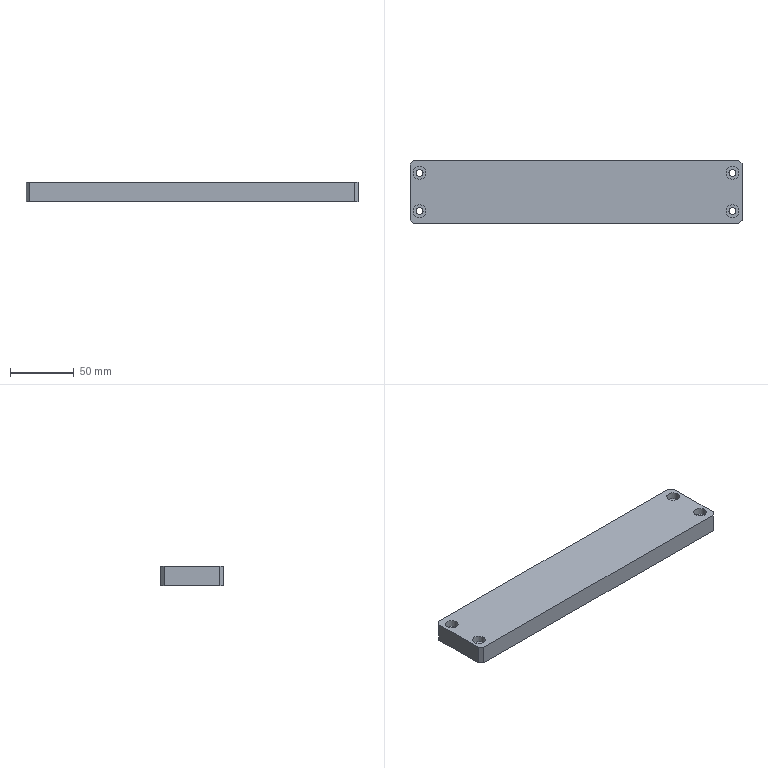Part | NX | 1 solid | 22 faces | box 261 x 50 x 15 mm | volume 192871 mm3 | plane 14 | cylinder 8 | commonest cylinder face diameters 5.5 x4 10 x4
STEP:
#1=CARTESIAN_POINT('',(-127.5,25.,7.5));
#2=VERTEX_POINT('',#1);
#3=CARTESIAN_POINT('',(-130.5,22.,7.5));
#4=VERTEX_POINT('',#3);
#5=CARTESIAN_POINT('',(-130.5,22.,7.5));
#6=DIRECTION('',(-0.7071,-0.7071,0.));
#7=VECTOR('',#6,1000.);
#8=LINE('',#5,#7);
#9=EDGE_CURVE('',#2,#4,#8,.T.);
#10=ORIENTED_EDGE('',*,*,#9,.F.);
#11=CARTESIAN_POINT('',(-127.5,25.,-7.5));
#12=VERTEX_POINT('',#11);
#13=CARTESIAN_POINT('',(-127.5,25.,7.5));
#14=DIRECTION('',(0.,0.,1.));
#15=VECTOR('',#14,1000.);
#16=LINE('',#13,#15);
#17=EDGE_CURVE('',#12,#2,#16,.T.);
#18=ORIENTED_EDGE('',*,*,#17,.F.);
#19=CARTESIAN_POINT('',(-130.5,22.,-7.5));
#20=VERTEX_POINT('',#19);
#21=CARTESIAN_POINT('',(-76.25,76.25,-7.5));
#22=DIRECTION('',(0.7071,0.7071,0.));
#23=VECTOR('',#22,1000.);
#24=LINE('',#21,#23);
#25=EDGE_CURVE('',#20,#12,#24,.T.);
#26=ORIENTED_EDGE('',*,*,#25,.F.);
#27=CARTESIAN_POINT('',(-130.5,22.,7.5));
#28=DIRECTION('',(0.,0.,-1.));
#29=VECTOR('',#28,1000.);
#30=LINE('',#27,#29);
#31=EDGE_CURVE('',#4,#20,#30,.T.);
#32=ORIENTED_EDGE('',*,*,#31,.F.);
#33=EDGE_LOOP('',(#10,#18,#26,#32));
#34=FACE_BOUND('',#33,.T.);
#35=CARTESIAN_POINT('',(-130.5,22.,7.5));
#36=DIRECTION('',(0.7071,-0.7071,0.));
#37=DIRECTION('',(0.,0.,-1.));
#38=AXIS2_PLACEMENT_3D('',#35,#36,#37);
#39=PLANE('',#38);
#40=ADVANCED_FACE('',(#34),#39,.F.);
#41=CARTESIAN_POINT('',(-130.5,-22.,7.5));
#42=VERTEX_POINT('',#41);
#43=CARTESIAN_POINT('',(-127.5,-25.,7.5));
#44=VERTEX_POINT('',#43);
#45=CARTESIAN_POINT('',(-127.5,-25.,7.5));
#46=DIRECTION('',(0.7071,-0.7071,0.));
#47=VECTOR('',#46,1000.);
#48=LINE('',#45,#47);
#49=EDGE_CURVE('',#42,#44,#48,.T.);
#50=ORIENTED_EDGE('',*,*,#49,.F.);
#51=CARTESIAN_POINT('',(-130.5,-22.,-7.5));
#52=VERTEX_POINT('',#51);
#53=CARTESIAN_POINT('',(-130.5,-22.,7.5));
#54=DIRECTION('',(0.,0.,1.));
#55=VECTOR('',#54,1000.);
#56=LINE('',#53,#55);
#57=EDGE_CURVE('',#52,#42,#56,.T.);
#58=ORIENTED_EDGE('',*,*,#57,.F.);
#59=CARTESIAN_POINT('',(-127.5,-25.,-7.5));
#60=VERTEX_POINT('',#59);
#61=CARTESIAN_POINT('',(-76.25,-76.25,-7.5));
#62=DIRECTION('',(-0.7071,0.7071,0.));
#63=VECTOR('',#62,1000.);
#64=LINE('',#61,#63);
#65=EDGE_CURVE('',#60,#52,#64,.T.);
#66=ORIENTED_EDGE('',*,*,#65,.F.);
#67=CARTESIAN_POINT('',(-127.5,-25.,-7.5));
#68=DIRECTION('',(0.,0.,-1.));
#69=VECTOR('',#68,1000.);
#70=LINE('',#67,#69);
#71=EDGE_CURVE('',#44,#60,#70,.T.);
#72=ORIENTED_EDGE('',*,*,#71,.F.);
#73=EDGE_LOOP('',(#50,#58,#66,#72));
#74=FACE_BOUND('',#73,.T.);
#75=CARTESIAN_POINT('',(-127.5,-25.,7.5));
#76=DIRECTION('',(-0.7071,-0.7071,0.));
#77=DIRECTION('',(0.,0.,1.));
#78=AXIS2_PLACEMENT_3D('',#75,#76,#77);
#79=PLANE('',#78);
#80=ADVANCED_FACE('',(#74),#79,.T.);
#81=CARTESIAN_POINT('',(130.5,22.,7.5));
#82=VERTEX_POINT('',#81);
#83=CARTESIAN_POINT('',(127.5,25.,7.5));
#84=VERTEX_POINT('',#83);
#85=CARTESIAN_POINT('',(127.5,25.,7.5));
#86=DIRECTION('',(-0.7071,0.7071,0.));
#87=VECTOR('',#86,1000.);
#88=LINE('',#85,#87);
#89=EDGE_CURVE('',#82,#84,#88,.T.);
#90=ORIENTED_EDGE('',*,*,#89,.F.);
#91=CARTESIAN_POINT('',(130.5,22.,-7.5));
#92=VERTEX_POINT('',#91);
#93=CARTESIAN_POINT('',(130.5,22.,7.5));
#94=DIRECTION('',(0.,0.,1.));
#95=VECTOR('',#94,1000.);
#96=LINE('',#93,#95);
#97=EDGE_CURVE('',#92,#82,#96,.T.);
#98=ORIENTED_EDGE('',*,*,#97,.F.);
#99=CARTESIAN_POINT('',(127.5,25.,-7.5));
#100=VERTEX_POINT('',#99);
#101=CARTESIAN_POINT('',(76.25,76.25,-7.5));
#102=DIRECTION('',(0.7071,-0.7071,0.));
#103=VECTOR('',#102,1000.);
#104=LINE('',#101,#103);
#105=EDGE_CURVE('',#100,#92,#104,.T.);
#106=ORIENTED_EDGE('',*,*,#105,.F.);
#107=CARTESIAN_POINT('',(127.5,25.,-7.5));
#108=DIRECTION('',(0.,0.,-1.));
#109=VECTOR('',#108,1000.);
#110=LINE('',#107,#109);
#111=EDGE_CURVE('',#84,#100,#110,.T.);
#112=ORIENTED_EDGE('',*,*,#111,.F.);
#113=EDGE_LOOP('',(#90,#98,#106,#112));
#114=FACE_BOUND('',#113,.T.);
#115=CARTESIAN_POINT('',(127.5,25.,7.5));
#116=DIRECTION('',(0.7071,0.7071,0.));
#117=DIRECTION('',(0.,0.,1.));
#118=AXIS2_PLACEMENT_3D('',#115,#116,#117);
#119=PLANE('',#118);
#120=ADVANCED_FACE('',(#114),#119,.T.);
#121=CARTESIAN_POINT('',(127.5,-25.,7.5));
#122=VERTEX_POINT('',#121);
#123=CARTESIAN_POINT('',(130.5,-22.,7.5));
#124=VERTEX_POINT('',#123);
#125=CARTESIAN_POINT('',(130.5,-22.,7.5));
#126=DIRECTION('',(0.7071,0.7071,0.));
#127=VECTOR('',#126,1000.);
#128=LINE('',#125,#127);
#129=EDGE_CURVE('',#122,#124,#128,.T.);
#130=ORIENTED_EDGE('',*,*,#129,.F.);
#131=CARTESIAN_POINT('',(127.5,-25.,-7.5));
#132=VERTEX_POINT('',#131);
#133=CARTESIAN_POINT('',(127.5,-25.,7.5));
#134=DIRECTION('',(0.,0.,1.));
#135=VECTOR('',#134,1000.);
#136=LINE('',#133,#135);
#137=EDGE_CURVE('',#132,#122,#136,.T.);
#138=ORIENTED_EDGE('',*,*,#137,.F.);
#139=CARTESIAN_POINT('',(130.5,-22.,-7.5));
#140=VERTEX_POINT('',#139);
#141=CARTESIAN_POINT('',(76.25,-76.25,-7.5));
#142=DIRECTION('',(-0.7071,-0.7071,0.));
#143=VECTOR('',#142,1000.);
#144=LINE('',#141,#143);
#145=EDGE_CURVE('',#140,#132,#144,.T.);
#146=ORIENTED_EDGE('',*,*,#145,.F.);
#147=CARTESIAN_POINT('',(130.5,-22.,7.5));
#148=DIRECTION('',(0.,0.,-1.));
#149=VECTOR('',#148,1000.);
#150=LINE('',#147,#149);
#151=EDGE_CURVE('',#124,#140,#150,.T.);
#152=ORIENTED_EDGE('',*,*,#151,.F.);
#153=EDGE_LOOP('',(#130,#138,#146,#152));
#154=FACE_BOUND('',#153,.T.);
#155=CARTESIAN_POINT('',(130.5,-22.,7.5));
#156=DIRECTION('',(-0.7071,0.7071,0.));
#157=DIRECTION('',(0.,0.,-1.));
#158=AXIS2_PLACEMENT_3D('',#155,#156,#157);
#159=PLANE('',#158);
#160=ADVANCED_FACE('',(#154),#159,.F.);
#161=CARTESIAN_POINT('',(128.,15.,2.1));
#162=VERTEX_POINT('',#161);
#163=CARTESIAN_POINT('',(123.,15.,2.1));
#164=DIRECTION('',(0.,0.,1.));
#165=DIRECTION('',(1.,0.,0.));
#166=AXIS2_PLACEMENT_3D('',#163,#164,#165);
#167=CIRCLE('',#166,5.);
#168=EDGE_CURVE('',#162,#162,#167,.T.);
#169=ORIENTED_EDGE('',*,*,#168,.T.);
#170=EDGE_LOOP('',(#169));
#171=FACE_BOUND('',#170,.T.);
#172=CARTESIAN_POINT('',(125.75,15.,2.1));
#173=VERTEX_POINT('',#172);
#174=CARTESIAN_POINT('',(123.,15.,2.1));
#175=DIRECTION('',(0.,0.,1.));
#176=DIRECTION('',(1.,0.,0.));
#177=AXIS2_PLACEMENT_3D('',#174,#175,#176);
#178=CIRCLE('',#177,2.75);
#179=EDGE_CURVE('',#173,#173,#178,.T.);
#180=ORIENTED_EDGE('',*,*,#179,.F.);
#181=EDGE_LOOP('',(#180));
#182=FACE_BOUND('',#181,.T.);
#183=CARTESIAN_POINT('',(125.75,15.,2.1));
#184=DIRECTION('',(0.,0.,-1.));
#185=DIRECTION('',(-1.,0.,0.));
#186=AXIS2_PLACEMENT_3D('',#183,#184,#185);
#187=PLANE('',#186);
#188=ADVANCED_FACE('',(#171,#182),#187,.F.);
#189=CARTESIAN_POINT('',(118.,-15.,2.1));
#190=VERTEX_POINT('',#189);
#191=CARTESIAN_POINT('',(123.,-15.,2.1));
#192=DIRECTION('',(0.,0.,1.));
#193=DIRECTION('',(-1.,0.,0.));
#194=AXIS2_PLACEMENT_3D('',#191,#192,#193);
#195=CIRCLE('',#194,5.);
#196=EDGE_CURVE('',#190,#190,#195,.T.);
#197=ORIENTED_EDGE('',*,*,#196,.T.);
#198=EDGE_LOOP('',(#197));
#199=FACE_BOUND('',#198,.T.);
#200=CARTESIAN_POINT('',(120.25,-15.,2.1));
#201=VERTEX_POINT('',#200);
#202=CARTESIAN_POINT('',(123.,-15.,2.1));
#203=DIRECTION('',(0.,0.,1.));
#204=DIRECTION('',(-1.,0.,0.));
#205=AXIS2_PLACEMENT_3D('',#202,#203,#204);
#206=CIRCLE('',#205,2.75);
#207=EDGE_CURVE('',#201,#201,#206,.T.);
#208=ORIENTED_EDGE('',*,*,#207,.F.);
#209=EDGE_LOOP('',(#208));
#210=FACE_BOUND('',#209,.T.);
#211=CARTESIAN_POINT('',(125.75,15.,2.1));
#212=DIRECTION('',(0.,0.,-1.));
#213=DIRECTION('',(-1.,0.,0.));
#214=AXIS2_PLACEMENT_3D('',#211,#212,#213);
#215=PLANE('',#214);
#216=ADVANCED_FACE('',(#199,#210),#215,.F.);
#217=CARTESIAN_POINT('',(-128.,15.,2.1));
#218=VERTEX_POINT('',#217);
#219=CARTESIAN_POINT('',(-123.,15.,2.1));
#220=DIRECTION('',(0.,0.,1.));
#221=DIRECTION('',(-1.,0.,0.));
#222=AXIS2_PLACEMENT_3D('',#219,#220,#221);
#223=CIRCLE('',#222,5.);
#224=EDGE_CURVE('',#218,#218,#223,.T.);
#225=ORIENTED_EDGE('',*,*,#224,.T.);
#226=EDGE_LOOP('',(#225));
#227=FACE_BOUND('',#226,.T.);
#228=CARTESIAN_POINT('',(-125.75,15.,2.1));
#229=VERTEX_POINT('',#228);
#230=CARTESIAN_POINT('',(-123.,15.,2.1));
#231=DIRECTION('',(0.,0.,1.));
#232=DIRECTION('',(-1.,0.,0.));
#233=AXIS2_PLACEMENT_3D('',#230,#231,#232);
#234=CIRCLE('',#233,2.75);
#235=EDGE_CURVE('',#229,#229,#234,.T.);
#236=ORIENTED_EDGE('',*,*,#235,.F.);
#237=EDGE_LOOP('',(#236));
#238=FACE_BOUND('',#237,.T.);
#239=CARTESIAN_POINT('',(125.75,15.,2.1));
#240=DIRECTION('',(0.,0.,-1.));
#241=DIRECTION('',(-1.,0.,0.));
#242=AXIS2_PLACEMENT_3D('',#239,#240,#241);
#243=PLANE('',#242);
#244=ADVANCED_FACE('',(#227,#238),#243,.F.);
#245=CARTESIAN_POINT('',(-128.,-15.,2.1));
#246=VERTEX_POINT('',#245);
#247=CARTESIAN_POINT('',(-123.,-15.,2.1));
#248=DIRECTION('',(0.,0.,1.));
#249=DIRECTION('',(-1.,0.,0.));
#250=AXIS2_PLACEMENT_3D('',#247,#248,#249);
#251=CIRCLE('',#250,5.);
#252=EDGE_CURVE('',#246,#246,#251,.T.);
#253=ORIENTED_EDGE('',*,*,#252,.T.);
#254=EDGE_LOOP('',(#253));
#255=FACE_BOUND('',#254,.T.);
#256=CARTESIAN_POINT('',(-125.75,-15.,2.1));
#257=VERTEX_POINT('',#256);
#258=CARTESIAN_POINT('',(-123.,-15.,2.1));
#259=DIRECTION('',(0.,0.,1.));
#260=DIRECTION('',(-1.,0.,0.));
#261=AXIS2_PLACEMENT_3D('',#258,#259,#260);
#262=CIRCLE('',#261,2.75);
#263=EDGE_CURVE('',#257,#257,#262,.T.);
#264=ORIENTED_EDGE('',*,*,#263,.F.);
#265=EDGE_LOOP('',(#264));
#266=FACE_BOUND('',#265,.T.);
#267=CARTESIAN_POINT('',(125.75,15.,2.1));
#268=DIRECTION('',(0.,0.,-1.));
#269=DIRECTION('',(-1.,0.,0.));
#270=AXIS2_PLACEMENT_3D('',#267,#268,#269);
#271=PLANE('',#270);
#272=ADVANCED_FACE('',(#255,#266),#271,.F.);
#273=CARTESIAN_POINT('',(130.5,-25.,-7.5));
#274=DIRECTION('',(0.,1.,0.));
#275=VECTOR('',#274,1000.);
#276=LINE('',#273,#275);
#277=EDGE_CURVE('',#140,#92,#276,.T.);
#278=ORIENTED_EDGE('',*,*,#277,.F.);
#279=ORIENTED_EDGE('',*,*,#145,.T.);
#280=CARTESIAN_POINT('',(-130.5,-25.,-7.5));
#281=DIRECTION('',(1.,0.,0.));
#282=VECTOR('',#281,1000.);
#283=LINE('',#280,#282);
#284=EDGE_CURVE('',#60,#132,#283,.T.);
#285=ORIENTED_EDGE('',*,*,#284,.F.);
#286=ORIENTED_EDGE('',*,*,#65,.T.);
#287=CARTESIAN_POINT('',(-130.5,-25.,-7.5));
#288=DIRECTION('',(0.,1.,0.));
#289=VECTOR('',#288,1000.);
#290=LINE('',#287,#289);
#291=EDGE_CURVE('',#52,#20,#290,.T.);
#292=ORIENTED_EDGE('',*,*,#291,.T.);
#293=ORIENTED_EDGE('',*,*,#25,.T.);
#294=CARTESIAN_POINT('',(-130.5,25.,-7.5));
#295=DIRECTION('',(1.,0.,0.));
#296=VECTOR('',#295,1000.);
#297=LINE('',#294,#296);
#298=EDGE_CURVE('',#12,#100,#297,.T.);
#299=ORIENTED_EDGE('',*,*,#298,.T.);
#300=ORIENTED_EDGE('',*,*,#105,.T.);
#301=EDGE_LOOP('',(#278,#279,#285,#286,#292,#293,#299,#300));
#302=FACE_BOUND('',#301,.T.);
#303=CARTESIAN_POINT('',(-120.25,-15.,-7.5));
#304=VERTEX_POINT('',#303);
#305=CARTESIAN_POINT('',(-123.,-15.,-7.5));
#306=DIRECTION('',(0.,0.,1.));
#307=DIRECTION('',(1.,0.,0.));
#308=AXIS2_PLACEMENT_3D('',#305,#306,#307);
#309=CIRCLE('',#308,2.75);
#310=EDGE_CURVE('',#304,#304,#309,.T.);
#311=ORIENTED_EDGE('',*,*,#310,.T.);
#312=EDGE_LOOP('',(#311));
#313=FACE_BOUND('',#312,.T.);
#314=CARTESIAN_POINT('',(-120.25,15.,-7.5));
#315=VERTEX_POINT('',#314);
#316=CARTESIAN_POINT('',(-123.,15.,-7.5));
#317=DIRECTION('',(0.,0.,1.));
#318=DIRECTION('',(1.,0.,0.));
#319=AXIS2_PLACEMENT_3D('',#316,#317,#318);
#320=CIRCLE('',#319,2.75);
#321=EDGE_CURVE('',#315,#315,#320,.T.);
#322=ORIENTED_EDGE('',*,*,#321,.T.);
#323=EDGE_LOOP('',(#322));
#324=FACE_BOUND('',#323,.T.);
#325=CARTESIAN_POINT('',(125.75,-15.,-7.5));
#326=VERTEX_POINT('',#325);
#327=CARTESIAN_POINT('',(123.,-15.,-7.5));
#328=DIRECTION('',(0.,0.,1.));
#329=DIRECTION('',(1.,0.,0.));
#330=AXIS2_PLACEMENT_3D('',#327,#328,#329);
#331=CIRCLE('',#330,2.75);
#332=EDGE_CURVE('',#326,#326,#331,.T.);
#333=ORIENTED_EDGE('',*,*,#332,.T.);
#334=EDGE_LOOP('',(#333));
#335=FACE_BOUND('',#334,.T.);
#336=CARTESIAN_POINT('',(125.75,15.,-7.5));
#337=VERTEX_POINT('',#336);
#338=CARTESIAN_POINT('',(123.,15.,-7.5));
#339=DIRECTION('',(0.,0.,1.));
#340=DIRECTION('',(1.,0.,0.));
#341=AXIS2_PLACEMENT_3D('',#338,#339,#340);
#342=CIRCLE('',#341,2.75);
#343=EDGE_CURVE('',#337,#337,#342,.T.);
#344=ORIENTED_EDGE('',*,*,#343,.T.);
#345=EDGE_LOOP('',(#344));
#346=FACE_BOUND('',#345,.T.);
#347=CARTESIAN_POINT('',(0.,0.,-7.5));
#348=DIRECTION('',(0.,0.,-1.));
#349=DIRECTION('',(-1.,0.,0.));
#350=AXIS2_PLACEMENT_3D('',#347,#348,#349);
#351=PLANE('',#350);
#352=ADVANCED_FACE('',(#302,#313,#324,#335,#346),#351,.T.);
#353=CARTESIAN_POINT('',(-130.5,-25.,7.5));
#354=DIRECTION('',(1.,0.,0.));
#355=VECTOR('',#354,1000.);
#356=LINE('',#353,#355);
#357=EDGE_CURVE('',#44,#122,#356,.T.);
#358=ORIENTED_EDGE('',*,*,#357,.T.);
#359=ORIENTED_EDGE('',*,*,#129,.T.);
#360=CARTESIAN_POINT('',(130.5,-25.,7.5));
#361=DIRECTION('',(0.,1.,0.));
#362=VECTOR('',#361,1000.);
#363=LINE('',#360,#362);
#364=EDGE_CURVE('',#124,#82,#363,.T.);
#365=ORIENTED_EDGE('',*,*,#364,.T.);
#366=ORIENTED_EDGE('',*,*,#89,.T.);
#367=CARTESIAN_POINT('',(-130.5,25.,7.5));
#368=DIRECTION('',(1.,0.,0.));
#369=VECTOR('',#368,1000.);
#370=LINE('',#367,#369);
#371=EDGE_CURVE('',#2,#84,#370,.T.);
#372=ORIENTED_EDGE('',*,*,#371,.F.);
#373=ORIENTED_EDGE('',*,*,#9,.T.);
#374=CARTESIAN_POINT('',(-130.5,-25.,7.5));
#375=DIRECTION('',(0.,1.,0.));
#376=VECTOR('',#375,1000.);
#377=LINE('',#374,#376);
#378=EDGE_CURVE('',#42,#4,#377,.T.);
#379=ORIENTED_EDGE('',*,*,#378,.F.);
#380=ORIENTED_EDGE('',*,*,#49,.T.);
#381=EDGE_LOOP('',(#358,#359,#365,#366,#372,#373,#379,#380));
#382=FACE_BOUND('',#381,.T.);
#383=CARTESIAN_POINT('',(-118.,-15.,7.5));
#384=VERTEX_POINT('',#383);
#385=CARTESIAN_POINT('',(-123.,-15.,7.5));
#386=DIRECTION('',(0.,0.,1.));
#387=DIRECTION('',(1.,0.,0.));
#388=AXIS2_PLACEMENT_3D('',#385,#386,#387);
#389=CIRCLE('',#388,5.);
#390=EDGE_CURVE('',#384,#384,#389,.T.);
#391=ORIENTED_EDGE('',*,*,#390,.F.);
#392=EDGE_LOOP('',(#391));
#393=FACE_BOUND('',#392,.T.);
#394=CARTESIAN_POINT('',(-118.,15.,7.5));
#395=VERTEX_POINT('',#394);
#396=CARTESIAN_POINT('',(-123.,15.,7.5));
#397=DIRECTION('',(0.,0.,1.));
#398=DIRECTION('',(1.,0.,0.));
#399=AXIS2_PLACEMENT_3D('',#396,#397,#398);
#400=CIRCLE('',#399,5.);
#401=EDGE_CURVE('',#395,#395,#400,.T.);
#402=ORIENTED_EDGE('',*,*,#401,.F.);
#403=EDGE_LOOP('',(#402));
#404=FACE_BOUND('',#403,.T.);
#405=CARTESIAN_POINT('',(128.,-15.,7.5));
#406=VERTEX_POINT('',#405);
#407=CARTESIAN_POINT('',(123.,-15.,7.5));
#408=DIRECTION('',(0.,0.,1.));
#409=DIRECTION('',(1.,0.,0.));
#410=AXIS2_PLACEMENT_3D('',#407,#408,#409);
#411=CIRCLE('',#410,5.);
#412=EDGE_CURVE('',#406,#406,#411,.T.);
#413=ORIENTED_EDGE('',*,*,#412,.F.);
#414=EDGE_LOOP('',(#413));
#415=FACE_BOUND('',#414,.T.);
#416=CARTESIAN_POINT('',(128.,15.,7.5));
#417=VERTEX_POINT('',#416);
#418=CARTESIAN_POINT('',(123.,15.,7.5));
#419=DIRECTION('',(0.,0.,1.));
#420=DIRECTION('',(1.,0.,0.));
#421=AXIS2_PLACEMENT_3D('',#418,#419,#420);
#422=CIRCLE('',#421,5.);
#423=EDGE_CURVE('',#417,#417,#422,.T.);
#424=ORIENTED_EDGE('',*,*,#423,.F.);
#425=EDGE_LOOP('',(#424));
#426=FACE_BOUND('',#425,.T.);
#427=CARTESIAN_POINT('',(0.,0.,7.5));
#428=DIRECTION('',(0.,0.,-1.));
#429=DIRECTION('',(-1.,0.,0.));
#430=AXIS2_PLACEMENT_3D('',#427,#428,#429);
#431=PLANE('',#430);
#432=ADVANCED_FACE('',(#382,#393,#404,#415,#426),#431,.F.);
#433=ORIENTED_EDGE('',*,*,#371,.T.);
#434=ORIENTED_EDGE('',*,*,#111,.T.);
#435=ORIENTED_EDGE('',*,*,#298,.F.);
#436=ORIENTED_EDGE('',*,*,#17,.T.);
#437=EDGE_LOOP('',(#433,#434,#435,#436));
#438=FACE_BOUND('',#437,.T.);
#439=CARTESIAN_POINT('',(-130.5,25.,7.5));
#440=DIRECTION('',(0.,1.,0.));
#441=DIRECTION('',(0.,0.,1.));
#442=AXIS2_PLACEMENT_3D('',#439,#440,#441);
#443=PLANE('',#442);
#444=ADVANCED_FACE('',(#438),#443,.T.);
#445=ORIENTED_EDGE('',*,*,#364,.F.);
#446=ORIENTED_EDGE('',*,*,#151,.T.);
#447=ORIENTED_EDGE('',*,*,#277,.T.);
#448=ORIENTED_EDGE('',*,*,#97,.T.);
#449=EDGE_LOOP('',(#445,#446,#447,#448));
#450=FACE_BOUND('',#449,.T.);
#451=CARTESIAN_POINT('',(130.5,-25.,7.5));
#452=DIRECTION('',(-1.,0.,0.));
#453=DIRECTION('',(0.,0.,1.));
#454=AXIS2_PLACEMENT_3D('',#451,#452,#453);
#455=PLANE('',#454);
#456=ADVANCED_FACE('',(#450),#455,.F.);
#457=ORIENTED_EDGE('',*,*,#284,.T.);
#458=ORIENTED_EDGE('',*,*,#137,.T.);
#459=ORIENTED_EDGE('',*,*,#357,.F.);
#460=ORIENTED_EDGE('',*,*,#71,.T.);
#461=EDGE_LOOP('',(#457,#458,#459,#460));
#462=FACE_BOUND('',#461,.T.);
#463=CARTESIAN_POINT('',(-130.5,-25.,7.5));
#464=DIRECTION('',(0.,1.,0.));
#465=DIRECTION('',(0.,0.,1.));
#466=AXIS2_PLACEMENT_3D('',#463,#464,#465);
#467=PLANE('',#466);
#468=ADVANCED_FACE('',(#462),#467,.F.);
#469=ORIENTED_EDGE('',*,*,#291,.F.);
#470=ORIENTED_EDGE('',*,*,#57,.T.);
#471=ORIENTED_EDGE('',*,*,#378,.T.);
#472=ORIENTED_EDGE('',*,*,#31,.T.);
#473=EDGE_LOOP('',(#469,#470,#471,#472));
#474=FACE_BOUND('',#473,.T.);
#475=CARTESIAN_POINT('',(-130.5,-25.,7.5));
#476=DIRECTION('',(-1.,0.,0.));
#477=DIRECTION('',(0.,0.,1.));
#478=AXIS2_PLACEMENT_3D('',#475,#476,#477);
#479=PLANE('',#478);
#480=ADVANCED_FACE('',(#474),#479,.T.);
#481=ORIENTED_EDGE('',*,*,#310,.F.);
#482=EDGE_LOOP('',(#481));
#483=FACE_BOUND('',#482,.T.);
#484=ORIENTED_EDGE('',*,*,#263,.T.);
#485=EDGE_LOOP('',(#484));
#486=FACE_BOUND('',#485,.T.);
#487=CARTESIAN_POINT('',(-123.,-15.,7.5));
#488=DIRECTION('',(0.,0.,1.));
#489=DIRECTION('',(1.,0.,0.));
#490=AXIS2_PLACEMENT_3D('',#487,#488,#489);
#491=CYLINDRICAL_SURFACE('',#490,2.75);
#492=ADVANCED_FACE('',(#483,#486),#491,.F.);
#493=ORIENTED_EDGE('',*,*,#252,.F.);
#494=EDGE_LOOP('',(#493));
#495=FACE_BOUND('',#494,.T.);
#496=ORIENTED_EDGE('',*,*,#390,.T.);
#497=EDGE_LOOP('',(#496));
#498=FACE_BOUND('',#497,.T.);
#499=CARTESIAN_POINT('',(-123.,-15.,7.5));
#500=DIRECTION('',(0.,0.,1.));
#501=DIRECTION('',(1.,0.,0.));
#502=AXIS2_PLACEMENT_3D('',#499,#500,#501);
#503=CYLINDRICAL_SURFACE('',#502,5.);
#504=ADVANCED_FACE('',(#495,#498),#503,.F.);
#505=ORIENTED_EDGE('',*,*,#321,.F.);
#506=EDGE_LOOP('',(#505));
#507=FACE_BOUND('',#506,.T.);
#508=ORIENTED_EDGE('',*,*,#235,.T.);
#509=EDGE_LOOP('',(#508));
#510=FACE_BOUND('',#509,.T.);
#511=CARTESIAN_POINT('',(-123.,15.,7.5));
#512=DIRECTION('',(0.,0.,1.));
#513=DIRECTION('',(1.,0.,0.));
#514=AXIS2_PLACEMENT_3D('',#511,#512,#513);
#515=CYLINDRICAL_SURFACE('',#514,2.75);
#516=ADVANCED_FACE('',(#507,#510),#515,.F.);
#517=ORIENTED_EDGE('',*,*,#224,.F.);
#518=EDGE_LOOP('',(#517));
#519=FACE_BOUND('',#518,.T.);
#520=ORIENTED_EDGE('',*,*,#401,.T.);
#521=EDGE_LOOP('',(#520));
#522=FACE_BOUND('',#521,.T.);
#523=CARTESIAN_POINT('',(-123.,15.,7.5));
#524=DIRECTION('',(0.,0.,1.));
#525=DIRECTION('',(1.,0.,0.));
#526=AXIS2_PLACEMENT_3D('',#523,#524,#525);
#527=CYLINDRICAL_SURFACE('',#526,5.);
#528=ADVANCED_FACE('',(#519,#522),#527,.F.);
#529=ORIENTED_EDGE('',*,*,#332,.F.);
#530=EDGE_LOOP('',(#529));
#531=FACE_BOUND('',#530,.T.);
#532=ORIENTED_EDGE('',*,*,#207,.T.);
#533=EDGE_LOOP('',(#532));
#534=FACE_BOUND('',#533,.T.);
#535=CARTESIAN_POINT('',(123.,-15.,7.5));
#536=DIRECTION('',(0.,0.,1.));
#537=DIRECTION('',(1.,0.,0.));
#538=AXIS2_PLACEMENT_3D('',#535,#536,#537);
#539=CYLINDRICAL_SURFACE('',#538,2.75);
#540=ADVANCED_FACE('',(#531,#534),#539,.F.);
#541=ORIENTED_EDGE('',*,*,#196,.F.);
#542=EDGE_LOOP('',(#541));
#543=FACE_BOUND('',#542,.T.);
#544=ORIENTED_EDGE('',*,*,#412,.T.);
#545=EDGE_LOOP('',(#544));
#546=FACE_BOUND('',#545,.T.);
#547=CARTESIAN_POINT('',(123.,-15.,7.5));
#548=DIRECTION('',(0.,0.,1.));
#549=DIRECTION('',(1.,0.,0.));
#550=AXIS2_PLACEMENT_3D('',#547,#548,#549);
#551=CYLINDRICAL_SURFACE('',#550,5.);
#552=ADVANCED_FACE('',(#543,#546),#551,.F.);
#553=ORIENTED_EDGE('',*,*,#343,.F.);
#554=EDGE_LOOP('',(#553));
#555=FACE_BOUND('',#554,.T.);
#556=ORIENTED_EDGE('',*,*,#179,.T.);
#557=EDGE_LOOP('',(#556));
#558=FACE_BOUND('',#557,.T.);
#559=CARTESIAN_POINT('',(123.,15.,7.5));
#560=DIRECTION('',(0.,0.,1.));
#561=DIRECTION('',(1.,0.,0.));
#562=AXIS2_PLACEMENT_3D('',#559,#560,#561);
#563=CYLINDRICAL_SURFACE('',#562,2.75);
#564=ADVANCED_FACE('',(#555,#558),#563,.F.);
#565=ORIENTED_EDGE('',*,*,#168,.F.);
#566=EDGE_LOOP('',(#565));
#567=FACE_BOUND('',#566,.T.);
#568=ORIENTED_EDGE('',*,*,#423,.T.);
#569=EDGE_LOOP('',(#568));
#570=FACE_BOUND('',#569,.T.);
#571=CARTESIAN_POINT('',(123.,15.,7.5));
#572=DIRECTION('',(0.,0.,1.));
#573=DIRECTION('',(1.,0.,0.));
#574=AXIS2_PLACEMENT_3D('',#571,#572,#573);
#575=CYLINDRICAL_SURFACE('',#574,5.);
#576=ADVANCED_FACE('',(#567,#570),#575,.F.);
#577=CLOSED_SHELL('',(#40,#80,#120,#160,#188,#216,#244,#272,#352,#432,#444,#456,#468,#480,#492,#504,#516,#528,#540,#552,#564,#576));
#578=MANIFOLD_SOLID_BREP('',#577);
#579=(LENGTH_UNIT()NAMED_UNIT(*)SI_UNIT(.MILLI.,.METRE.));
#580=UNCERTAINTY_MEASURE_WITH_UNIT(LENGTH_MEASURE(0.00001),#579,'','');
#581=(NAMED_UNIT(*)PLANE_ANGLE_UNIT()SI_UNIT($,.RADIAN.));
#582=(NAMED_UNIT(*)SI_UNIT($,.STERADIAN.)SOLID_ANGLE_UNIT());
#583=(GEOMETRIC_REPRESENTATION_CONTEXT(3)GLOBAL_UNCERTAINTY_ASSIGNED_CONTEXT((#580))GLOBAL_UNIT_ASSIGNED_CONTEXT((#579,#581,#582))REPRESENTATION_CONTEXT('',''));
#584=ADVANCED_BREP_SHAPE_REPRESENTATION('',(#578),#583);